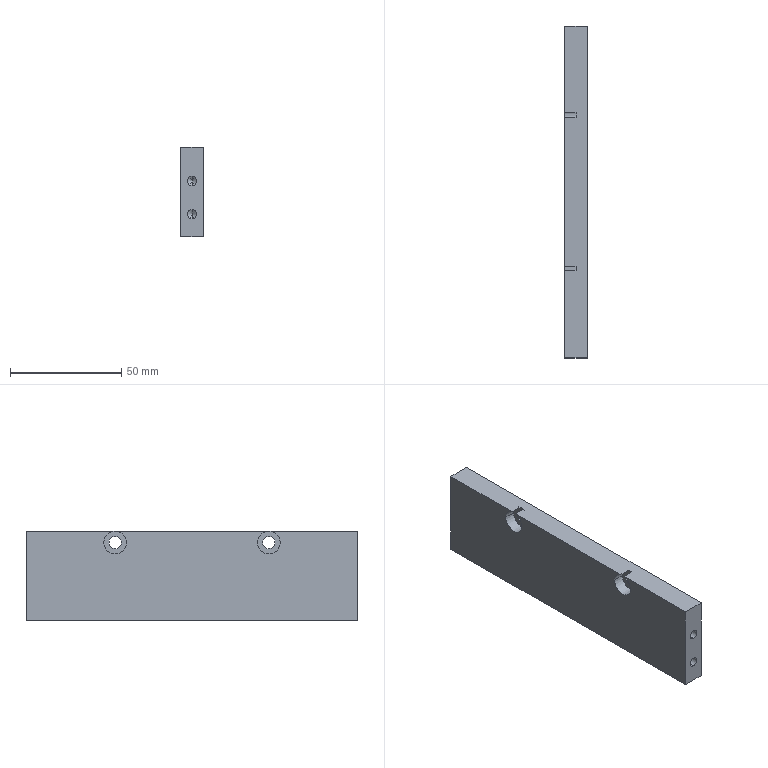Part | STEP file | 05-09 Fixing connection plate 1 | 1 solid | 34 faces | box 10 x 149 x 40 mm | volume 57725 mm3 | cylinder 18 | cone 8 | plane 8 | commonest cylinder face diameters 4.2 x8 10.2 x6 5.5 x4